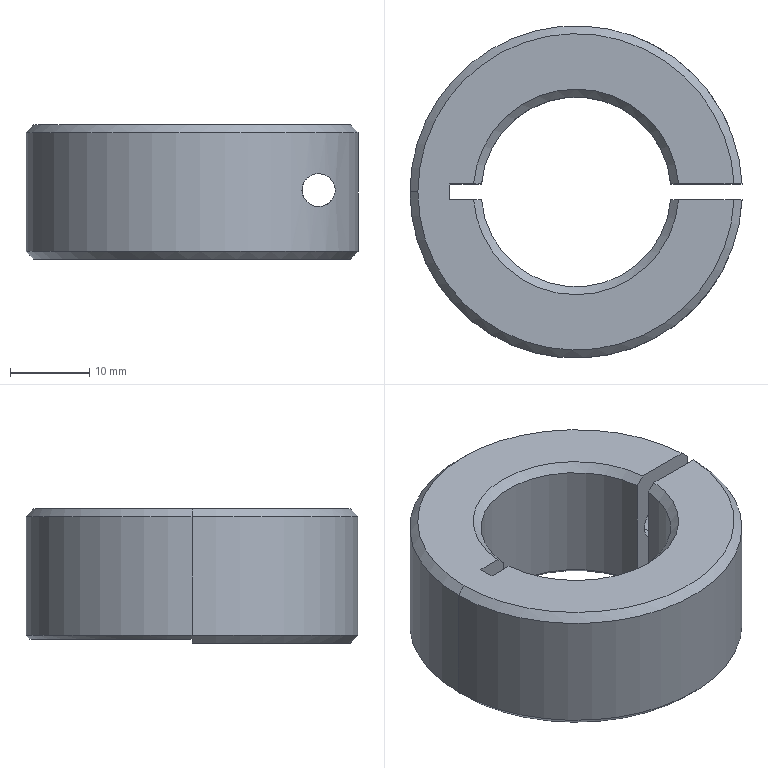Part | SolidWorks | features ICE 7, Chamfer 2, HoleWzd 2 | 1 solid | 44 faces | box 41.976 x 42 x 17 mm | volume 13853 mm3 | cylinder 18 | cone 13 | plane 13 | commonest cylinder face diameters 3.3 x6 14 x3 4.2 x2 5.5 x2 24 x2 42 x2
STEP:
#1=CARTESIAN_POINT('',(15.988,13.615,1.75));
#2=VERTEX_POINT('',#1);
#3=CARTESIAN_POINT('',(15.988,13.615,15.75));
#4=VERTEX_POINT('',#3);
#5=CARTESIAN_POINT('',(15.988,13.615,1.75));
#6=CARTESIAN_POINT('',(15.646,14.017,1.75));
#7=CARTESIAN_POINT('',(15.292,14.403,1.775));
#8=CARTESIAN_POINT('',(14.558,15.144,1.888));
#9=CARTESIAN_POINT('',(14.178,15.5,1.976));
#10=CARTESIAN_POINT('',(13.402,16.176,2.232));
#11=CARTESIAN_POINT('',(13.014,16.489,2.398));
#12=CARTESIAN_POINT('',(12.437,16.923,2.714));
#13=CARTESIAN_POINT('',(12.245,17.062,2.83));
#14=CARTESIAN_POINT('',(11.866,17.328,3.088));
#15=CARTESIAN_POINT('',(11.678,17.455,3.229));
#16=CARTESIAN_POINT('',(11.137,17.809,3.681));
#17=CARTESIAN_POINT('',(10.8,18.013,4.024));
#18=CARTESIAN_POINT('',(10.34,18.279,4.608));
#19=CARTESIAN_POINT('',(10.193,18.361,4.815));
#20=CARTESIAN_POINT('',(9.922,18.509,5.247));
#21=CARTESIAN_POINT('',(9.799,18.574,5.47));
#22=CARTESIAN_POINT('',(9.576,18.69,5.931));
#23=CARTESIAN_POINT('',(9.476,18.74,6.168));
#24=CARTESIAN_POINT('',(9.303,18.827,6.658));
#25=CARTESIAN_POINT('',(9.229,18.864,6.912));
#26=CARTESIAN_POINT('',(9.05,18.95,7.683));
#27=CARTESIAN_POINT('',(8.989,18.979,8.204));
#28=CARTESIAN_POINT('',(8.987,18.98,8.998));
#29=CARTESIAN_POINT('',(9.002,18.973,9.266));
#30=CARTESIAN_POINT('',(9.061,18.945,9.791));
#31=CARTESIAN_POINT('',(9.105,18.924,10.049));
#32=CARTESIAN_POINT('',(9.221,18.867,10.559));
#33=CARTESIAN_POINT('',(9.293,18.832,10.811));
#34=CARTESIAN_POINT('',(9.466,18.746,11.306));
#35=CARTESIAN_POINT('',(9.566,18.695,11.548));
#36=CARTESIAN_POINT('',(9.9,18.521,12.243));
#37=CARTESIAN_POINT('',(10.17,18.376,12.675));
#38=CARTESIAN_POINT('',(10.789,18.02,13.464));
#39=CARTESIAN_POINT('',(11.129,17.814,13.811));
#40=CARTESIAN_POINT('',(11.672,17.459,14.266));
#41=CARTESIAN_POINT('',(11.86,17.332,14.408));
#42=CARTESIAN_POINT('',(12.239,17.066,14.666));
#43=CARTESIAN_POINT('',(12.43,16.928,14.783));
#44=CARTESIAN_POINT('',(12.816,16.637,14.994));
#45=CARTESIAN_POINT('',(13.01,16.486,15.089));
#46=CARTESIAN_POINT('',(13.4,16.171,15.257));
#47=CARTESIAN_POINT('',(13.596,16.006,15.332));
#48=CARTESIAN_POINT('',(14.565,15.163,15.652));
#49=CARTESIAN_POINT('',(15.301,14.422,15.75));
#50=CARTESIAN_POINT('',(15.988,13.615,15.75));
#51=B_SPLINE_CURVE_WITH_KNOTS('',3,(#5,#6,#7,#8,#9,#10,#11,#12,#13,#14,#15,#16,#17,#18,#19,#20,#21,#22,#23,#24,#25,#26,#27,#28,#29,#30,#31,#32,#33,#34,#35,#36,#37,#38,#39,#40,#41,#42,#43,#44,#45,#46,#47,#48,#49,#50),.UNSPECIFIED.,.F.,.F.,(4,2,2,2,2,2,2,2,2,2,2,2,2,2,2,2,2,2,2,2,2,2,4),(0.0005356,0.002108,0.00368,0.005253,0.006039,0.006825,0.008398,0.009184,0.00997,0.01076,0.01154,0.01311,0.0139,0.01469,0.01547,0.01626,0.01783,0.0194,0.02019,0.02098,0.02176,0.02255,0.02569),.UNSPECIFIED.);
#52=EDGE_CURVE('',#2,#4,#51,.T.);
#53=ORIENTED_EDGE('',*,*,#52,.T.);
#54=CARTESIAN_POINT('',(15.988,13.2,15.75));
#55=VERTEX_POINT('',#54);
#56=CARTESIAN_POINT('',(15.988,30.2,15.75));
#57=DIRECTION('',(0.,-1.,0.));
#58=VECTOR('',#57,1000.);
#59=LINE('',#56,#58);
#60=EDGE_CURVE('',#4,#55,#59,.T.);
#61=ORIENTED_EDGE('',*,*,#60,.T.);
#62=CARTESIAN_POINT('',(15.988,13.2,1.75));
#63=VERTEX_POINT('',#62);
#64=CARTESIAN_POINT('',(15.988,13.2,8.75));
#65=DIRECTION('',(0.,1.,0.));
#66=DIRECTION('',(0.,0.,1.));
#67=AXIS2_PLACEMENT_3D('',#64,#65,#66);
#68=CIRCLE('',#67,7.);
#69=EDGE_CURVE('',#63,#55,#68,.T.);
#70=ORIENTED_EDGE('',*,*,#69,.F.);
#71=CARTESIAN_POINT('',(15.988,30.2,1.75));
#72=DIRECTION('',(0.,-1.,0.));
#73=VECTOR('',#72,1000.);
#74=LINE('',#71,#73);
#75=EDGE_CURVE('',#2,#63,#74,.T.);
#76=ORIENTED_EDGE('',*,*,#75,.F.);
#77=EDGE_LOOP('',(#53,#61,#70,#76));
#78=FACE_OUTER_BOUND('',#77,.T.);
#79=CARTESIAN_POINT('',(15.988,30.2,8.75));
#80=DIRECTION('',(0.,-1.,0.));
#81=DIRECTION('',(0.,0.,-1.));
#82=AXIS2_PLACEMENT_3D('',#79,#80,#81);
#83=CYLINDRICAL_SURFACE('',#82,7.);
#84=ADVANCED_FACE('',(#78),#83,.F.);
#85=CARTESIAN_POINT('',(16.333,13.2,1.758));
#86=VERTEX_POINT('',#85);
#87=CARTESIAN_POINT('',(16.333,13.2,1.758));
#88=CARTESIAN_POINT('',(16.219,13.34,1.753));
#89=CARTESIAN_POINT('',(16.104,13.479,1.75));
#90=CARTESIAN_POINT('',(15.988,13.615,1.75));
#91=B_SPLINE_CURVE_WITH_KNOTS('',3,(#87,#88,#89,#90),.UNSPECIFIED.,.F.,.F.,(4,4),(0.,0.0005356),.UNSPECIFIED.);
#92=EDGE_CURVE('',#86,#2,#91,.T.);
#93=ORIENTED_EDGE('',*,*,#92,.T.);
#94=ORIENTED_EDGE('',*,*,#75,.T.);
#95=CARTESIAN_POINT('',(15.988,13.2,8.75));
#96=DIRECTION('',(0.,1.,0.));
#97=DIRECTION('',(0.,0.,1.));
#98=AXIS2_PLACEMENT_3D('',#95,#96,#97);
#99=CIRCLE('',#98,7.);
#100=EDGE_CURVE('',#86,#63,#99,.T.);
#101=ORIENTED_EDGE('',*,*,#100,.F.);
#102=EDGE_LOOP('',(#93,#94,#101));
#103=FACE_OUTER_BOUND('',#102,.T.);
#104=CARTESIAN_POINT('',(15.988,30.2,8.75));
#105=DIRECTION('',(0.,-1.,0.));
#106=DIRECTION('',(0.,0.,-1.));
#107=AXIS2_PLACEMENT_3D('',#104,#105,#106);
#108=CYLINDRICAL_SURFACE('',#107,7.);
#109=ADVANCED_FACE('',(#103),#108,.F.);
#110=CARTESIAN_POINT('',(-14.795,-5.985,10.1));
#111=VERTEX_POINT('',#110);
#112=CARTESIAN_POINT('',(-18.095,-5.985,10.1));
#113=VERTEX_POINT('',#112);
#114=CARTESIAN_POINT('',(-16.445,-5.985,10.1));
#115=DIRECTION('',(0.,0.,-1.));
#116=DIRECTION('',(-1.,0.,0.));
#117=AXIS2_PLACEMENT_3D('',#114,#115,#116);
#118=CIRCLE('',#117,1.65);
#119=EDGE_CURVE('',#111,#113,#118,.T.);
#120=ORIENTED_EDGE('',*,*,#119,.F.);
#121=CARTESIAN_POINT('',(-14.795,-5.985,0.));
#122=VERTEX_POINT('',#121);
#123=CARTESIAN_POINT('',(-14.795,-5.985,0.));
#124=DIRECTION('',(0.,0.,-1.));
#125=VECTOR('',#124,1000.);
#126=LINE('',#123,#125);
#127=EDGE_CURVE('',#111,#122,#126,.T.);
#128=ORIENTED_EDGE('',*,*,#127,.T.);
#129=CARTESIAN_POINT('',(-18.095,-5.985,0.));
#130=VERTEX_POINT('',#129);
#131=CARTESIAN_POINT('',(-16.445,-5.985,0.));
#132=DIRECTION('',(0.,0.,-1.));
#133=DIRECTION('',(-1.,0.,0.));
#134=AXIS2_PLACEMENT_3D('',#131,#132,#133);
#135=CIRCLE('',#134,1.65);
#136=EDGE_CURVE('',#122,#130,#135,.T.);
#137=ORIENTED_EDGE('',*,*,#136,.T.);
#138=CARTESIAN_POINT('',(-18.095,-5.985,0.));
#139=DIRECTION('',(0.,0.,-1.));
#140=VECTOR('',#139,1000.);
#141=LINE('',#138,#140);
#142=EDGE_CURVE('',#113,#130,#141,.T.);
#143=ORIENTED_EDGE('',*,*,#142,.F.);
#144=EDGE_LOOP('',(#120,#128,#137,#143));
#145=FACE_OUTER_BOUND('',#144,.T.);
#146=CARTESIAN_POINT('',(-16.445,-5.985,0.));
#147=DIRECTION('',(0.,0.,-1.));
#148=DIRECTION('',(-1.,0.,0.));
#149=AXIS2_PLACEMENT_3D('',#146,#147,#148);
#150=CYLINDRICAL_SURFACE('',#149,1.65);
#151=ADVANCED_FACE('',(#145),#150,.F.);
#152=CARTESIAN_POINT('',(-16.445,-5.985,11.091));
#153=VERTEX_POINT('',#152);
#154=CARTESIAN_POINT('',(-18.095,-5.985,10.1));
#155=DIRECTION('',(-0.8572,0.,-0.515));
#156=VECTOR('',#155,1000.);
#157=LINE('',#154,#156);
#158=EDGE_CURVE('',#153,#113,#157,.T.);
#159=ORIENTED_EDGE('',*,*,#158,.F.);
#160=CARTESIAN_POINT('',(-14.795,-5.985,10.1));
#161=DIRECTION('',(0.8572,0.,-0.515));
#162=VECTOR('',#161,1000.);
#163=LINE('',#160,#162);
#164=EDGE_CURVE('',#153,#111,#163,.T.);
#165=ORIENTED_EDGE('',*,*,#164,.T.);
#166=ORIENTED_EDGE('',*,*,#119,.T.);
#167=EDGE_LOOP('',(#159,#165,#166));
#168=FACE_OUTER_BOUND('',#167,.T.);
#169=CARTESIAN_POINT('',(-16.445,-5.985,10.1));
#170=DIRECTION('',(0.,0.,-1.));
#171=DIRECTION('',(-1.,0.,0.));
#172=AXIS2_PLACEMENT_3D('',#169,#170,#171);
#173=CONICAL_SURFACE('',#172,1.65,1.03);
#174=ADVANCED_FACE('',(#168),#173,.F.);
#175=CARTESIAN_POINT('',(10.4,-15.155,10.1));
#176=VERTEX_POINT('',#175);
#177=CARTESIAN_POINT('',(7.1,-15.155,10.1));
#178=VERTEX_POINT('',#177);
#179=CARTESIAN_POINT('',(8.75,-15.155,10.1));
#180=DIRECTION('',(0.,0.,-1.));
#181=DIRECTION('',(-1.,0.,0.));
#182=AXIS2_PLACEMENT_3D('',#179,#180,#181);
#183=CIRCLE('',#182,1.65);
#184=EDGE_CURVE('',#176,#178,#183,.T.);
#185=ORIENTED_EDGE('',*,*,#184,.F.);
#186=CARTESIAN_POINT('',(10.4,-15.155,0.));
#187=VERTEX_POINT('',#186);
#188=CARTESIAN_POINT('',(10.4,-15.155,0.));
#189=DIRECTION('',(0.,0.,-1.));
#190=VECTOR('',#189,1000.);
#191=LINE('',#188,#190);
#192=EDGE_CURVE('',#176,#187,#191,.T.);
#193=ORIENTED_EDGE('',*,*,#192,.T.);
#194=CARTESIAN_POINT('',(7.1,-15.155,0.));
#195=VERTEX_POINT('',#194);
#196=CARTESIAN_POINT('',(8.75,-15.155,0.));
#197=DIRECTION('',(0.,0.,-1.));
#198=DIRECTION('',(-1.,0.,0.));
#199=AXIS2_PLACEMENT_3D('',#196,#197,#198);
#200=CIRCLE('',#199,1.65);
#201=EDGE_CURVE('',#187,#195,#200,.T.);
#202=ORIENTED_EDGE('',*,*,#201,.T.);
#203=CARTESIAN_POINT('',(7.1,-15.155,0.));
#204=DIRECTION('',(0.,0.,-1.));
#205=VECTOR('',#204,1000.);
#206=LINE('',#203,#205);
#207=EDGE_CURVE('',#178,#195,#206,.T.);
#208=ORIENTED_EDGE('',*,*,#207,.F.);
#209=EDGE_LOOP('',(#185,#193,#202,#208));
#210=FACE_OUTER_BOUND('',#209,.T.);
#211=CARTESIAN_POINT('',(8.75,-15.155,0.));
#212=DIRECTION('',(0.,0.,-1.));
#213=DIRECTION('',(-1.,0.,0.));
#214=AXIS2_PLACEMENT_3D('',#211,#212,#213);
#215=CYLINDRICAL_SURFACE('',#214,1.65);
#216=ADVANCED_FACE('',(#210),#215,.F.);
#217=CARTESIAN_POINT('',(8.75,-15.155,11.091));
#218=VERTEX_POINT('',#217);
#219=CARTESIAN_POINT('',(7.1,-15.155,10.1));
#220=DIRECTION('',(-0.8572,0.,-0.515));
#221=VECTOR('',#220,1000.);
#222=LINE('',#219,#221);
#223=EDGE_CURVE('',#218,#178,#222,.T.);
#224=ORIENTED_EDGE('',*,*,#223,.F.);
#225=CARTESIAN_POINT('',(10.4,-15.155,10.1));
#226=DIRECTION('',(0.8572,0.,-0.515));
#227=VECTOR('',#226,1000.);
#228=LINE('',#225,#227);
#229=EDGE_CURVE('',#218,#176,#228,.T.);
#230=ORIENTED_EDGE('',*,*,#229,.T.);
#231=ORIENTED_EDGE('',*,*,#184,.T.);
#232=EDGE_LOOP('',(#224,#230,#231));
#233=FACE_OUTER_BOUND('',#232,.T.);
#234=CARTESIAN_POINT('',(8.75,-15.155,10.1));
#235=DIRECTION('',(0.,0.,-1.));
#236=DIRECTION('',(-1.,0.,0.));
#237=AXIS2_PLACEMENT_3D('',#234,#235,#236);
#238=CONICAL_SURFACE('',#237,1.65,1.03);
#239=ADVANCED_FACE('',(#233),#238,.F.);
#240=CARTESIAN_POINT('',(-4.335,-16.445,10.1));
#241=VERTEX_POINT('',#240);
#242=CARTESIAN_POINT('',(-7.635,-16.445,10.1));
#243=VERTEX_POINT('',#242);
#244=CARTESIAN_POINT('',(-5.985,-16.445,10.1));
#245=DIRECTION('',(0.,0.,-1.));
#246=DIRECTION('',(-1.,0.,0.));
#247=AXIS2_PLACEMENT_3D('',#244,#245,#246);
#248=CIRCLE('',#247,1.65);
#249=EDGE_CURVE('',#241,#243,#248,.T.);
#250=ORIENTED_EDGE('',*,*,#249,.F.);
#251=CARTESIAN_POINT('',(-4.335,-16.445,0.));
#252=VERTEX_POINT('',#251);
#253=CARTESIAN_POINT('',(-4.335,-16.445,0.));
#254=DIRECTION('',(0.,0.,-1.));
#255=VECTOR('',#254,1000.);
#256=LINE('',#253,#255);
#257=EDGE_CURVE('',#241,#252,#256,.T.);
#258=ORIENTED_EDGE('',*,*,#257,.T.);
#259=CARTESIAN_POINT('',(-7.635,-16.445,0.));
#260=VERTEX_POINT('',#259);
#261=CARTESIAN_POINT('',(-5.985,-16.445,0.));
#262=DIRECTION('',(0.,0.,-1.));
#263=DIRECTION('',(-1.,0.,0.));
#264=AXIS2_PLACEMENT_3D('',#261,#262,#263);
#265=CIRCLE('',#264,1.65);
#266=EDGE_CURVE('',#252,#260,#265,.T.);
#267=ORIENTED_EDGE('',*,*,#266,.T.);
#268=CARTESIAN_POINT('',(-7.635,-16.445,0.));
#269=DIRECTION('',(0.,0.,-1.));
#270=VECTOR('',#269,1000.);
#271=LINE('',#268,#270);
#272=EDGE_CURVE('',#243,#260,#271,.T.);
#273=ORIENTED_EDGE('',*,*,#272,.F.);
#274=EDGE_LOOP('',(#250,#258,#267,#273));
#275=FACE_OUTER_BOUND('',#274,.T.);
#276=CARTESIAN_POINT('',(-5.985,-16.445,0.));
#277=DIRECTION('',(0.,0.,-1.));
#278=DIRECTION('',(-1.,0.,0.));
#279=AXIS2_PLACEMENT_3D('',#276,#277,#278);
#280=CYLINDRICAL_SURFACE('',#279,1.65);
#281=ADVANCED_FACE('',(#275),#280,.F.);
#282=CARTESIAN_POINT('',(-5.985,-16.445,11.091));
#283=VERTEX_POINT('',#282);
#284=CARTESIAN_POINT('',(-7.635,-16.445,10.1));
#285=DIRECTION('',(-0.8572,0.,-0.515));
#286=VECTOR('',#285,1000.);
#287=LINE('',#284,#286);
#288=EDGE_CURVE('',#283,#243,#287,.T.);
#289=ORIENTED_EDGE('',*,*,#288,.F.);
#290=CARTESIAN_POINT('',(-4.335,-16.445,10.1));
#291=DIRECTION('',(0.8572,0.,-0.515));
#292=VECTOR('',#291,1000.);
#293=LINE('',#290,#292);
#294=EDGE_CURVE('',#283,#241,#293,.T.);
#295=ORIENTED_EDGE('',*,*,#294,.T.);
#296=ORIENTED_EDGE('',*,*,#249,.T.);
#297=EDGE_LOOP('',(#289,#295,#296));
#298=FACE_OUTER_BOUND('',#297,.T.);
#299=CARTESIAN_POINT('',(-5.985,-16.445,10.1));
#300=DIRECTION('',(0.,0.,-1.));
#301=DIRECTION('',(-1.,0.,0.));
#302=AXIS2_PLACEMENT_3D('',#299,#300,#301);
#303=CONICAL_SURFACE('',#302,1.65,1.03);
#304=ADVANCED_FACE('',(#298),#303,.F.);
#305=CARTESIAN_POINT('',(15.988,-13.615,6.65));
#306=VERTEX_POINT('',#305);
#307=CARTESIAN_POINT('',(15.988,-13.615,10.85));
#308=VERTEX_POINT('',#307);
#309=CARTESIAN_POINT('',(15.988,-13.615,6.65));
#310=CARTESIAN_POINT('',(15.769,-13.873,6.65));
#311=CARTESIAN_POINT('',(15.546,-14.122,6.683));
#312=CARTESIAN_POINT('',(15.21,-14.481,6.796));
#313=CARTESIAN_POINT('',(15.096,-14.599,6.845));
#314=CARTESIAN_POINT('',(14.875,-14.824,6.965));
#315=CARTESIAN_POINT('',(14.767,-14.931,7.036));
#316=CARTESIAN_POINT('',(14.454,-15.237,7.291));
#317=CARTESIAN_POINT('',(14.26,-15.417,7.516));
#318=CARTESIAN_POINT('',(14.046,-15.611,7.935));
#319=CARTESIAN_POINT('',(13.989,-15.662,8.085));
#320=CARTESIAN_POINT('',(13.909,-15.733,8.41));
#321=CARTESIAN_POINT('',(13.888,-15.752,8.576));
#322=CARTESIAN_POINT('',(13.888,-15.752,8.915));
#323=CARTESIAN_POINT('',(13.908,-15.734,9.085));
#324=CARTESIAN_POINT('',(13.987,-15.664,9.407));
#325=CARTESIAN_POINT('',(14.045,-15.613,9.561));
#326=CARTESIAN_POINT('',(14.187,-15.484,9.84));
#327=CARTESIAN_POINT('',(14.271,-15.406,9.968));
#328=CARTESIAN_POINT('',(14.455,-15.234,10.192));
#329=CARTESIAN_POINT('',(14.555,-15.138,10.291));
#330=CARTESIAN_POINT('',(14.87,-14.832,10.548));
#331=CARTESIAN_POINT('',(15.092,-14.606,10.664));
#332=CARTESIAN_POINT('',(15.544,-14.124,10.816));
#333=CARTESIAN_POINT('',(15.768,-13.874,10.85));
#334=CARTESIAN_POINT('',(15.988,-13.615,10.85));
#335=B_SPLINE_CURVE_WITH_KNOTS('',3,(#309,#310,#311,#312,#313,#314,#315,#316,#317,#318,#319,#320,#321,#322,#323,#324,#325,#326,#327,#328,#329,#330,#331,#332,#333,#334),.UNSPECIFIED.,.F.,.F.,(4,2,2,2,2,2,2,2,2,2,2,2,4),(0.009008,0.01001,0.01052,0.01102,0.01202,0.01253,0.01303,0.01353,0.01403,0.01453,0.01504,0.01604,0.01705),.UNSPECIFIED.);
#336=EDGE_CURVE('',#306,#308,#335,.T.);
#337=ORIENTED_EDGE('',*,*,#336,.F.);
#338=CARTESIAN_POINT('',(15.988,-1.,6.65));
#339=VERTEX_POINT('',#338);
#340=CARTESIAN_POINT('',(15.988,-1.,6.65));
#341=DIRECTION('',(0.,1.,0.));
#342=VECTOR('',#341,1000.);
#343=LINE('',#340,#342);
#344=EDGE_CURVE('',#306,#339,#343,.T.);
#345=ORIENTED_EDGE('',*,*,#344,.T.);
#346=CARTESIAN_POINT('',(15.988,-1.,10.85));
#347=VERTEX_POINT('',#346);
#348=CARTESIAN_POINT('',(15.988,-1.,8.75));
#349=DIRECTION('',(0.,1.,0.));
#350=DIRECTION('',(0.,0.,1.));
#351=AXIS2_PLACEMENT_3D('',#348,#349,#350);
#352=CIRCLE('',#351,2.1);
#353=EDGE_CURVE('',#339,#347,#352,.T.);
#354=ORIENTED_EDGE('',*,*,#353,.T.);
#355=CARTESIAN_POINT('',(15.988,-1.,10.85));
#356=DIRECTION('',(0.,1.,0.));
#357=VECTOR('',#356,1000.);
#358=LINE('',#355,#357);
#359=EDGE_CURVE('',#308,#347,#358,.T.);
#360=ORIENTED_EDGE('',*,*,#359,.F.);
#361=EDGE_LOOP('',(#337,#345,#354,#360));
#362=FACE_OUTER_BOUND('',#361,.T.);
#363=CARTESIAN_POINT('',(15.988,-1.,8.75));
#364=DIRECTION('',(0.,1.,0.));
#365=DIRECTION('',(0.,0.,1.));
#366=AXIS2_PLACEMENT_3D('',#363,#364,#365);
#367=CYLINDRICAL_SURFACE('',#366,2.1);
#368=ADVANCED_FACE('',(#362),#367,.F.);
#369=CARTESIAN_POINT('',(15.988,9.,6.));
#370=VERTEX_POINT('',#369);
#371=CARTESIAN_POINT('',(15.988,9.,11.5));
#372=VERTEX_POINT('',#371);
#373=CARTESIAN_POINT('',(15.988,9.,8.75));
#374=DIRECTION('',(0.,1.,0.));
#375=DIRECTION('',(0.,0.,-1.));
#376=AXIS2_PLACEMENT_3D('',#373,#374,#375);
#377=CIRCLE('',#376,2.75);
#378=EDGE_CURVE('',#370,#372,#377,.T.);
#379=ORIENTED_EDGE('',*,*,#378,.T.);
#380=CARTESIAN_POINT('',(15.988,1.,11.5));
#381=VERTEX_POINT('',#380);
#382=CARTESIAN_POINT('',(15.988,31.,11.5));
#383=DIRECTION('',(0.,-1.,0.));
#384=VECTOR('',#383,1000.);
#385=LINE('',#382,#384);
#386=EDGE_CURVE('',#372,#381,#385,.T.);
#387=ORIENTED_EDGE('',*,*,#386,.T.);
#388=CARTESIAN_POINT('',(15.988,1.,6.));
#389=VERTEX_POINT('',#388);
#390=CARTESIAN_POINT('',(15.988,1.,8.75));
#391=DIRECTION('',(0.,-1.,0.));
#392=DIRECTION('',(0.,0.,-1.));
#393=AXIS2_PLACEMENT_3D('',#390,#391,#392);
#394=CIRCLE('',#393,2.75);
#395=EDGE_CURVE('',#381,#389,#394,.T.);
#396=ORIENTED_EDGE('',*,*,#395,.T.);
#397=CARTESIAN_POINT('',(15.988,31.,6.));
#398=DIRECTION('',(0.,-1.,0.));
#399=VECTOR('',#398,1000.);
#400=LINE('',#397,#399);
#401=EDGE_CURVE('',#370,#389,#400,.T.);
#402=ORIENTED_EDGE('',*,*,#401,.F.);
#403=EDGE_LOOP('',(#379,#387,#396,#402));
#404=FACE_OUTER_BOUND('',#403,.T.);
#405=CARTESIAN_POINT('',(15.988,31.,8.75));
#406=DIRECTION('',(0.,-1.,0.));
#407=DIRECTION('',(0.,0.,-1.));
#408=AXIS2_PLACEMENT_3D('',#405,#406,#407);
#409=CYLINDRICAL_SURFACE('',#408,2.75);
#410=ADVANCED_FACE('',(#404),#409,.F.);
#411=CARTESIAN_POINT('',(-20.,0.,17.));
#412=VERTEX_POINT('',#411);
#413=CARTESIAN_POINT('',(19.975,-1.,17.));
#414=VERTEX_POINT('',#413);
#415=CARTESIAN_POINT('',(0.,0.,17.));
#416=DIRECTION('',(0.,0.,1.));
#417=DIRECTION('',(1.,0.,0.));
#418=AXIS2_PLACEMENT_3D('',#415,#416,#417);
#419=CIRCLE('',#418,20.);
#420=EDGE_CURVE('',#412,#414,#419,.T.);
#421=ORIENTED_EDGE('',*,*,#420,.F.);
#422=CARTESIAN_POINT('',(-21.,0.,16.));
#423=VERTEX_POINT('',#422);
#424=CARTESIAN_POINT('',(-20.,0.,17.));
#425=DIRECTION('',(-0.7071,0.,-0.7071));
#426=VECTOR('',#425,1000.);
#427=LINE('',#424,#426);
#428=EDGE_CURVE('',#412,#423,#427,.T.);
#429=ORIENTED_EDGE('',*,*,#428,.T.);
#430=CARTESIAN_POINT('',(20.976,-1.,16.));
#431=VERTEX_POINT('',#430);
#432=CARTESIAN_POINT('',(0.,0.,16.));
#433=DIRECTION('',(0.,0.,-1.));
#434=DIRECTION('',(1.,0.,0.));
#435=AXIS2_PLACEMENT_3D('',#432,#433,#434);
#436=CIRCLE('',#435,21.);
#437=EDGE_CURVE('',#431,#423,#436,.T.);
#438=ORIENTED_EDGE('',*,*,#437,.F.);
#439=CARTESIAN_POINT('',(19.975,-1.,17.));
#440=CARTESIAN_POINT('',(20.309,-1.,16.667));
#441=CARTESIAN_POINT('',(20.642,-1.,16.333));
#442=CARTESIAN_POINT('',(20.976,-1.,16.));
#443=B_SPLINE_CURVE_WITH_KNOTS('',3,(#439,#440,#441,#442),.UNSPECIFIED.,.F.,.F.,(4,4),(0.08115,0.08257),.UNSPECIFIED.);
#444=EDGE_CURVE('',#414,#431,#443,.T.);
#445=ORIENTED_EDGE('',*,*,#444,.F.);
#446=EDGE_LOOP('',(#421,#429,#438,#445));
#447=FACE_OUTER_BOUND('',#446,.T.);
#448=CARTESIAN_POINT('',(0.,0.,17.));
#449=DIRECTION('',(0.,0.,-1.));
#450=DIRECTION('',(-1.,0.,0.));
#451=AXIS2_PLACEMENT_3D('',#448,#449,#450);
#452=CONICAL_SURFACE('',#451,20.,0.7854);
#453=ADVANCED_FACE('',(#447),#452,.T.);
#454=CARTESIAN_POINT('',(15.988,-13.615,10.85));
#455=CARTESIAN_POINT('',(16.235,-13.326,10.85));
#456=CARTESIAN_POINT('',(16.469,-13.035,10.808));
#457=CARTESIAN_POINT('',(16.915,-12.451,10.649));
#458=CARTESIAN_POINT('',(17.129,-12.154,10.531));
#459=CARTESIAN_POINT('',(17.419,-11.731,10.292));
#460=CARTESIAN_POINT('',(17.511,-11.593,10.202));
#461=CARTESIAN_POINT('',(17.685,-11.326,9.995));
#462=CARTESIAN_POINT('',(17.766,-11.198,9.878));
#463=CARTESIAN_POINT('',(17.909,-10.968,9.612));
#464=CARTESIAN_POINT('',(17.971,-10.865,9.462));
#465=CARTESIAN_POINT('',(18.062,-10.714,9.125));
#466=CARTESIAN_POINT('',(18.089,-10.668,8.935));
#467=CARTESIAN_POINT('',(18.088,-10.67,8.554));
#468=CARTESIAN_POINT('',(18.06,-10.717,8.366));
#469=CARTESIAN_POINT('',(17.969,-10.869,8.031));
#470=CARTESIAN_POINT('',(17.906,-10.973,7.881));
#471=CARTESIAN_POINT('',(17.763,-11.203,7.617));
#472=CARTESIAN_POINT('',(17.681,-11.332,7.5));
#473=CARTESIAN_POINT('',(17.508,-11.597,7.295));
#474=CARTESIAN_POINT('',(17.416,-11.735,7.205));
#475=CARTESIAN_POINT('',(17.223,-12.016,7.047));
#476=CARTESIAN_POINT('',(17.121,-12.161,6.978));
#477=CARTESIAN_POINT('',(16.91,-12.453,6.86));
#478=CARTESIAN_POINT('',(16.802,-12.598,6.811));
#479=CARTESIAN_POINT('',(16.469,-13.035,6.692));
#480=CARTESIAN_POINT('',(16.234,-13.327,6.65));
#481=CARTESIAN_POINT('',(15.988,-13.615,6.65));
#482=B_SPLINE_CURVE_WITH_KNOTS('',3,(#454,#455,#456,#457,#458,#459,#460,#461,#462,#463,#464,#465,#466,#467,#468,#469,#470,#471,#472,#473,#474,#475,#476,#477,#478,#479,#480,#481),.UNSPECIFIED.,.F.,.F.,(4,2,2,2,2,2,2,2,2,2,2,2,2,4),(0.,0.001126,0.002252,0.002815,0.003378,0.003941,0.004504,0.005067,0.00563,0.006193,0.006756,0.007319,0.007882,0.009008),.UNSPECIFIED.);
#483=EDGE_CURVE('',#308,#306,#482,.T.);
#484=ORIENTED_EDGE('',*,*,#483,.T.);
#485=ORIENTED_EDGE('',*,*,#336,.T.);
#486=EDGE_LOOP('',(#484,#485));
#487=FACE_BOUND('',#486,.T.);
#488=ORIENTED_EDGE('',*,*,#437,.T.);
#489=CARTESIAN_POINT('',(-21.,0.,1.));
#490=VERTEX_POINT('',#489);
#491=CARTESIAN_POINT('',(-21.,0.,17.));
#492=DIRECTION('',(0.,0.,-1.));
#493=VECTOR('',#492,1000.);
#494=LINE('',#491,#493);
#495=EDGE_CURVE('',#423,#490,#494,.T.);
#496=ORIENTED_EDGE('',*,*,#495,.T.);
#497=CARTESIAN_POINT('',(20.976,-1.,1.));
#498=VERTEX_POINT('',#497);
#499=CARTESIAN_POINT('',(0.,0.,1.));
#500=DIRECTION('',(0.,0.,1.));
#501=DIRECTION('',(1.,0.,0.));
#502=AXIS2_PLACEMENT_3D('',#499,#500,#501);
#503=CIRCLE('',#502,21.);
#504=EDGE_CURVE('',#490,#498,#503,.T.);
#505=ORIENTED_EDGE('',*,*,#504,.T.);
#506=CARTESIAN_POINT('',(20.976,-1.,17.));
#507=DIRECTION('',(0.,0.,1.));
#508=VECTOR('',#507,1000.);
#509=LINE('',#506,#508);
#510=EDGE_CURVE('',#498,#431,#509,.T.);
#511=ORIENTED_EDGE('',*,*,#510,.T.);
#512=EDGE_LOOP('',(#488,#496,#505,#511));
#513=FACE_OUTER_BOUND('',#512,.T.);
#514=CARTESIAN_POINT('',(0.,0.,17.));
#515=DIRECTION('',(0.,0.,-1.));
#516=DIRECTION('',(-1.,0.,0.));
#517=AXIS2_PLACEMENT_3D('',#514,#515,#516);
#518=CYLINDRICAL_SURFACE('',#517,21.);
#519=ADVANCED_FACE('',(#487,#513),#518,.T.);
#520=ORIENTED_EDGE('',*,*,#495,.F.);
#521=CARTESIAN_POINT('',(20.976,1.,16.));
#522=VERTEX_POINT('',#521);
#523=CARTESIAN_POINT('',(0.,0.,16.));
#524=DIRECTION('',(0.,0.,-1.));
#525=DIRECTION('',(1.,0.,0.));
#526=AXIS2_PLACEMENT_3D('',#523,#524,#525);
#527=CIRCLE('',#526,21.);
#528=EDGE_CURVE('',#423,#522,#527,.T.);
#529=ORIENTED_EDGE('',*,*,#528,.T.);
#530=CARTESIAN_POINT('',(20.976,1.,1.));
#531=VERTEX_POINT('',#530);
#532=CARTESIAN_POINT('',(20.976,1.,17.));
#533=DIRECTION('',(0.,0.,-1.));
#534=VECTOR('',#533,1000.);
#535=LINE('',#532,#534);
#536=EDGE_CURVE('',#522,#531,#535,.T.);
#537=ORIENTED_EDGE('',*,*,#536,.T.);
#538=CARTESIAN_POINT('',(0.,0.,1.));
#539=DIRECTION('',(0.,0.,1.));
#540=DIRECTION('',(1.,0.,0.));
#541=AXIS2_PLACEMENT_3D('',#538,#539,#540);
#542=CIRCLE('',#541,21.);
#543=EDGE_CURVE('',#531,#490,#542,.T.);
#544=ORIENTED_EDGE('',*,*,#543,.T.);
#545=EDGE_LOOP('',(#520,#529,#537,#544));
#546=FACE_OUTER_BOUND('',#545,.T.);
#547=CARTESIAN_POINT('',(16.333,13.2,15.742));
#548=VERTEX_POINT('',#547);
#549=CARTESIAN_POINT('',(16.333,13.2,14.5));
#550=VERTEX_POINT('',#549);
#551=CARTESIAN_POINT('',(16.333,13.2,17.));
#552=DIRECTION('',(0.,0.,-1.));
#553=VECTOR('',#552,1000.);
#554=LINE('',#551,#553);
#555=EDGE_CURVE('',#548,#550,#554,.T.);
#556=ORIENTED_EDGE('',*,*,#555,.F.);
#557=CARTESIAN_POINT('',(15.988,13.615,15.75));
#558=CARTESIAN_POINT('',(16.105,13.479,15.75));
#559=CARTESIAN_POINT('',(16.22,13.34,15.747));
#560=CARTESIAN_POINT('',(16.333,13.2,15.742));
#561=B_SPLINE_CURVE_WITH_KNOTS('',3,(#557,#558,#559,#560),.UNSPECIFIED.,.F.,.F.,(4,4),(0.02569,0.02623),.UNSPECIFIED.);
#562=EDGE_CURVE('',#4,#548,#561,.T.);
#563=ORIENTED_EDGE('',*,*,#562,.F.);
#564=ORIENTED_EDGE('',*,*,#52,.F.);
#565=ORIENTED_EDGE('',*,*,#92,.F.);
#566=CARTESIAN_POINT('',(16.333,13.2,3.));
#567=VERTEX_POINT('',#566);
#568=CARTESIAN_POINT('',(16.333,13.2,17.));
#569=DIRECTION('',(0.,0.,-1.));
#570=VECTOR('',#569,1000.);
#571=LINE('',#568,#570);
#572=EDGE_CURVE('',#567,#86,#571,.T.);
#573=ORIENTED_EDGE('',*,*,#572,.F.);
#574=CARTESIAN_POINT('',(18.974,9.,3.));
#575=VERTEX_POINT('',#574);
#576=CARTESIAN_POINT('',(0.,0.,3.));
#577=DIRECTION('',(0.,0.,-1.));
#578=DIRECTION('',(-1.,0.,0.));
#579=AXIS2_PLACEMENT_3D('',#576,#577,#578);
#580=CIRCLE('',#579,21.);
#581=EDGE_CURVE('',#567,#575,#580,.T.);
#582=ORIENTED_EDGE('',*,*,#581,.T.);
#583=CARTESIAN_POINT('',(18.974,9.,14.5));
#584=VERTEX_POINT('',#583);
#585=CARTESIAN_POINT('',(18.974,9.,17.));
#586=DIRECTION('',(0.,0.,1.));
#587=VECTOR('',#586,1000.);
#588=LINE('',#585,#587);
#589=EDGE_CURVE('',#575,#584,#588,.T.);
#590=ORIENTED_EDGE('',*,*,#589,.T.);
#591=CARTESIAN_POINT('',(0.,0.,14.5));
#592=DIRECTION('',(0.,0.,1.));
#593=DIRECTION('',(1.,0.,0.));
#594=AXIS2_PLACEMENT_3D('',#591,#592,#593);
#595=CIRCLE('',#594,21.);
#596=EDGE_CURVE('',#584,#550,#595,.T.);
#597=ORIENTED_EDGE('',*,*,#596,.T.);
#598=EDGE_LOOP('',(#556,#563,#564,#565,#573,#582,#590,#597));
#599=FACE_BOUND('',#598,.T.);
#600=CARTESIAN_POINT('',(0.,0.,17.));
#601=DIRECTION('',(0.,0.,-1.));
#602=DIRECTION('',(-1.,0.,0.));
#603=AXIS2_PLACEMENT_3D('',#600,#601,#602);
#604=CYLINDRICAL_SURFACE('',#603,21.);
#605=ADVANCED_FACE('',(#546,#599),#604,.T.);
#606=CARTESIAN_POINT('',(15.988,13.2,3.));
#607=VERTEX_POINT('',#606);
#608=CARTESIAN_POINT('',(20.976,13.2,3.));
#609=DIRECTION('',(1.,0.,0.));
#610=VECTOR('',#609,1000.);
#611=LINE('',#608,#610);
#612=EDGE_CURVE('',#607,#567,#611,.T.);
#613=ORIENTED_EDGE('',*,*,#612,.F.);
#614=CARTESIAN_POINT('',(15.988,9.,3.));
#615=VERTEX_POINT('',#614);
#616=CARTESIAN_POINT('',(15.988,39.,3.));
#617=DIRECTION('',(0.,-1.,0.));
#618=VECTOR('',#617,1000.);
#619=LINE('',#616,#618);
#620=EDGE_CURVE('',#607,#615,#619,.T.);
#621=ORIENTED_EDGE('',*,*,#620,.T.);
#622=CARTESIAN_POINT('',(20.976,9.,3.));
#623=DIRECTION('',(1.,0.,0.));
#624=VECTOR('',#623,1000.);
#625=LINE('',#622,#624);
#626=EDGE_CURVE('',#615,#575,#625,.T.);
#627=ORIENTED_EDGE('',*,*,#626,.T.);
#628=ORIENTED_EDGE('',*,*,#581,.F.);
#629=EDGE_LOOP('',(#613,#621,#627,#628));
#630=FACE_OUTER_BOUND('',#629,.T.);
#631=CARTESIAN_POINT('',(20.976,39.,3.));
#632=DIRECTION('',(0.,0.,-1.));
#633=DIRECTION('',(-1.,0.,0.));
#634=AXIS2_PLACEMENT_3D('',#631,#632,#633);
#635=PLANE('',#634);
#636=ADVANCED_FACE('',(#630),#635,.F.);
#637=CARTESIAN_POINT('',(15.988,13.2,14.5));
#638=VERTEX_POINT('',#637);
#639=CARTESIAN_POINT('',(15.988,13.2,8.75));
#640=DIRECTION('',(0.,-1.,0.));
#641=DIRECTION('',(0.,0.,1.));
#642=AXIS2_PLACEMENT_3D('',#639,#640,#641);
#643=CIRCLE('',#642,5.75);
#644=EDGE_CURVE('',#638,#607,#643,.T.);
#645=ORIENTED_EDGE('',*,*,#644,.F.);
#646=CARTESIAN_POINT('',(15.988,9.,14.5));
#647=VERTEX_POINT('',#646);
#648=CARTESIAN_POINT('',(15.988,39.,14.5));
#649=DIRECTION('',(0.,-1.,0.));
#650=VECTOR('',#649,1000.);
#651=LINE('',#648,#650);
#652=EDGE_CURVE('',#638,#647,#651,.T.);
#653=ORIENTED_EDGE('',*,*,#652,.T.);
#654=CARTESIAN_POINT('',(15.988,9.,8.75));
#655=DIRECTION('',(0.,-1.,0.));
#656=DIRECTION('',(0.,0.,-1.));
#657=AXIS2_PLACEMENT_3D('',#654,#655,#656);
#658=CIRCLE('',#657,5.75);
#659=EDGE_CURVE('',#647,#615,#658,.T.);
#660=ORIENTED_EDGE('',*,*,#659,.T.);
#661=ORIENTED_EDGE('',*,*,#620,.F.);
#662=EDGE_LOOP('',(#645,#653,#660,#661));
#663=FACE_OUTER_BOUND('',#662,.T.);
#664=CARTESIAN_POINT('',(15.988,39.,8.75));
#665=DIRECTION('',(0.,-1.,0.));
#666=DIRECTION('',(0.,0.,-1.));
#667=AXIS2_PLACEMENT_3D('',#664,#665,#666);
#668=CYLINDRICAL_SURFACE('',#667,5.75);
#669=ADVANCED_FACE('',(#663),#668,.F.);
#670=CARTESIAN_POINT('',(15.988,13.2,14.5));
#671=DIRECTION('',(-1.,0.,0.));
#672=VECTOR('',#671,1000.);
#673=LINE('',#670,#672);
#674=EDGE_CURVE('',#550,#638,#673,.T.);
#675=ORIENTED_EDGE('',*,*,#674,.F.);
#676=ORIENTED_EDGE('',*,*,#596,.F.);
#677=CARTESIAN_POINT('',(15.988,9.,14.5));
#678=DIRECTION('',(-1.,0.,0.));
#679=VECTOR('',#678,1000.);
#680=LINE('',#677,#679);
#681=EDGE_CURVE('',#584,#647,#680,.T.);
#682=ORIENTED_EDGE('',*,*,#681,.T.);
#683=ORIENTED_EDGE('',*,*,#652,.F.);
#684=EDGE_LOOP('',(#675,#676,#682,#683));
#685=FACE_OUTER_BOUND('',#684,.T.);
#686=CARTESIAN_POINT('',(15.988,39.,14.5));
#687=DIRECTION('',(0.,0.,1.));
#688=DIRECTION('',(1.,0.,0.));
#689=AXIS2_PLACEMENT_3D('',#686,#687,#688);
#690=PLANE('',#689);
#691=ADVANCED_FACE('',(#685),#690,.F.);
#692=CARTESIAN_POINT('',(11.958,1.,16.));
#693=VERTEX_POINT('',#692);
#694=CARTESIAN_POINT('',(11.958,1.,1.));
#695=VERTEX_POINT('',#694);
#696=CARTESIAN_POINT('',(11.958,1.,17.));
#697=DIRECTION('',(0.,0.,-1.));
#698=VECTOR('',#697,1000.);
#699=LINE('',#696,#698);
#700=EDGE_CURVE('',#693,#695,#699,.T.);
#701=ORIENTED_EDGE('',*,*,#700,.F.);
#702=CARTESIAN_POINT('',(-11.958,1.,16.));
#703=VERTEX_POINT('',#702);
#704=CARTESIAN_POINT('',(0.,0.,16.));
#705=DIRECTION('',(0.,0.,1.));
#706=DIRECTION('',(1.,0.,0.));
#707=AXIS2_PLACEMENT_3D('',#704,#705,#706);
#708=CIRCLE('',#707,12.);
#709=EDGE_CURVE('',#693,#703,#708,.T.);
#710=ORIENTED_EDGE('',*,*,#709,.T.);
#711=CARTESIAN_POINT('',(-11.958,1.,1.));
#712=VERTEX_POINT('',#711);
#713=CARTESIAN_POINT('',(-11.958,1.,17.));
#714=DIRECTION('',(0.,0.,1.));
#715=VECTOR('',#714,1000.);
#716=LINE('',#713,#715);
#717=EDGE_CURVE('',#712,#703,#716,.T.);
#718=ORIENTED_EDGE('',*,*,#717,.F.);
#719=CARTESIAN_POINT('',(0.,0.,1.));
#720=DIRECTION('',(0.,0.,-1.));
#721=DIRECTION('',(1.,0.,0.));
#722=AXIS2_PLACEMENT_3D('',#719,#720,#721);
#723=CIRCLE('',#722,12.);
#724=EDGE_CURVE('',#712,#695,#723,.T.);
#725=ORIENTED_EDGE('',*,*,#724,.T.);
#726=EDGE_LOOP('',(#701,#710,#718,#725));
#727=FACE_OUTER_BOUND('',#726,.T.);
#728=CARTESIAN_POINT('',(0.,0.,17.));
#729=DIRECTION('',(0.,0.,-1.));
#730=DIRECTION('',(-1.,0.,0.));
#731=AXIS2_PLACEMENT_3D('',#728,#729,#730);
#732=CYLINDRICAL_SURFACE('',#731,12.);
#733=ADVANCED_FACE('',(#727),#732,.F.);
#734=CARTESIAN_POINT('',(12.961,1.,17.));
#735=VERTEX_POINT('',#734);
#736=CARTESIAN_POINT('',(12.961,1.,17.));
#737=CARTESIAN_POINT('',(12.627,1.,16.667));
#738=CARTESIAN_POINT('',(12.293,1.,16.333));
#739=CARTESIAN_POINT('',(11.958,1.,16.));
#740=B_SPLINE_CURVE_WITH_KNOTS('',3,(#736,#737,#738,#739),.UNSPECIFIED.,.F.,.F.,(4,4),(0.02209,0.02351),.UNSPECIFIED.);
#741=EDGE_CURVE('',#735,#693,#740,.T.);
#742=ORIENTED_EDGE('',*,*,#741,.F.);
#743=CARTESIAN_POINT('',(-12.961,1.,17.));
#744=VERTEX_POINT('',#743);
#745=CARTESIAN_POINT('',(0.,0.,17.));
#746=DIRECTION('',(0.,0.,-1.));
#747=DIRECTION('',(1.,0.,0.));
#748=AXIS2_PLACEMENT_3D('',#745,#746,#747);
#749=CIRCLE('',#748,13.);
#750=EDGE_CURVE('',#744,#735,#749,.T.);
#751=ORIENTED_EDGE('',*,*,#750,.F.);
#752=CARTESIAN_POINT('',(-11.958,1.,16.));
#753=CARTESIAN_POINT('',(-12.293,1.,16.333));
#754=CARTESIAN_POINT('',(-12.627,1.,16.667));
#755=CARTESIAN_POINT('',(-12.961,1.,17.));
#756=B_SPLINE_CURVE_WITH_KNOTS('',3,(#752,#753,#754,#755),.UNSPECIFIED.,.F.,.F.,(4,4),(0.05622,0.05764),.UNSPECIFIED.);
#757=EDGE_CURVE('',#703,#744,#756,.T.);
#758=ORIENTED_EDGE('',*,*,#757,.F.);
#759=ORIENTED_EDGE('',*,*,#709,.F.);
#760=EDGE_LOOP('',(#742,#751,#758,#759));
#761=FACE_OUTER_BOUND('',#760,.T.);
#762=CARTESIAN_POINT('',(0.,0.,16.));
#763=DIRECTION('',(0.,0.,1.));
#764=DIRECTION('',(1.,0.,0.));
#765=AXIS2_PLACEMENT_3D('',#762,#763,#764);
#766=CONICAL_SURFACE('',#765,12.,0.7854);
#767=ADVANCED_FACE('',(#761),#766,.F.);
#768=CARTESIAN_POINT('',(12.46,1.,0.5));
#769=VERTEX_POINT('',#768);
#770=CARTESIAN_POINT('',(-12.46,1.,0.5));
#771=VERTEX_POINT('',#770);
#772=CARTESIAN_POINT('',(0.,0.,0.5));
#773=DIRECTION('',(0.,0.,1.));
#774=DIRECTION('',(1.,0.,0.));
#775=AXIS2_PLACEMENT_3D('',#772,#773,#774);
#776=CIRCLE('',#775,12.5);
#777=EDGE_CURVE('',#769,#771,#776,.T.);
#778=ORIENTED_EDGE('',*,*,#777,.F.);
#779=CARTESIAN_POINT('',(11.958,1.,1.));
#780=CARTESIAN_POINT('',(12.125,1.,0.8333));
#781=CARTESIAN_POINT('',(12.293,1.,0.6667));
#782=CARTESIAN_POINT('',(12.46,1.,0.5));
#783=B_SPLINE_CURVE_WITH_KNOTS('',3,(#779,#780,#781,#782),.UNSPECIFIED.,.F.,.F.,(4,4),(0.05622,0.05693),.UNSPECIFIED.);
#784=EDGE_CURVE('',#695,#769,#783,.T.);
#785=ORIENTED_EDGE('',*,*,#784,.F.);
#786=ORIENTED_EDGE('',*,*,#724,.F.);
#787=CARTESIAN_POINT('',(-12.46,1.,0.5));
#788=CARTESIAN_POINT('',(-12.293,1.,0.6667));
#789=CARTESIAN_POINT('',(-12.125,1.,0.8333));
#790=CARTESIAN_POINT('',(-11.958,1.,1.));
#791=B_SPLINE_CURVE_WITH_KNOTS('',3,(#787,#788,#789,#790),.UNSPECIFIED.,.F.,.F.,(4,4),(0.0228,0.02351),.UNSPECIFIED.);
#792=EDGE_CURVE('',#771,#712,#791,.T.);
#793=ORIENTED_EDGE('',*,*,#792,.F.);
#794=EDGE_LOOP('',(#778,#785,#786,#793));
#795=FACE_OUTER_BOUND('',#794,.T.);
#796=CARTESIAN_POINT('',(0.,0.,0.));
#797=DIRECTION('',(0.,0.,-1.));
#798=DIRECTION('',(-1.,0.,0.));
#799=AXIS2_PLACEMENT_3D('',#796,#797,#798);
#800=CONICAL_SURFACE('',#799,13.,0.7854);
#801=ADVANCED_FACE('',(#795),#800,.F.);
#802=CARTESIAN_POINT('',(19.975,1.,17.));
#803=VERTEX_POINT('',#802);
#804=CARTESIAN_POINT('',(-16.,1.,17.));
#805=DIRECTION('',(-1.,0.,0.));
#806=VECTOR('',#805,1000.);
#807=LINE('',#804,#806);
#808=EDGE_CURVE('',#803,#735,#807,.T.);
#809=ORIENTED_EDGE('',*,*,#808,.F.);
#810=CARTESIAN_POINT('',(0.,0.,17.));
#811=DIRECTION('',(0.,0.,1.));
#812=DIRECTION('',(1.,0.,0.));
#813=AXIS2_PLACEMENT_3D('',#810,#811,#812);
#814=CIRCLE('',#813,20.);
#815=EDGE_CURVE('',#803,#412,#814,.T.);
#816=ORIENTED_EDGE('',*,*,#815,.T.);
#817=ORIENTED_EDGE('',*,*,#420,.T.);
#818=CARTESIAN_POINT('',(12.961,-1.,17.));
#819=VERTEX_POINT('',#818);
#820=CARTESIAN_POINT('',(-16.,-1.,17.));
#821=DIRECTION('',(1.,0.,0.));
#822=VECTOR('',#821,1000.);
#823=LINE('',#820,#822);
#824=EDGE_CURVE('',#819,#414,#823,.T.);
#825=ORIENTED_EDGE('',*,*,#824,.F.);
#826=CARTESIAN_POINT('',(-12.961,-1.,17.));
#827=VERTEX_POINT('',#826);
#828=CARTESIAN_POINT('',(0.,0.,17.));
#829=DIRECTION('',(0.,0.,-1.));
#830=DIRECTION('',(1.,0.,0.));
#831=AXIS2_PLACEMENT_3D('',#828,#829,#830);
#832=CIRCLE('',#831,13.);
#833=EDGE_CURVE('',#819,#827,#832,.T.);
#834=ORIENTED_EDGE('',*,*,#833,.T.);
#835=CARTESIAN_POINT('',(-16.,-1.,17.));
#836=VERTEX_POINT('',#835);
#837=CARTESIAN_POINT('',(-16.,-1.,17.));
#838=DIRECTION('',(1.,0.,0.));
#839=VECTOR('',#838,1000.);
#840=LINE('',#837,#839);
#841=EDGE_CURVE('',#836,#827,#840,.T.);
#842=ORIENTED_EDGE('',*,*,#841,.F.);
#843=CARTESIAN_POINT('',(-16.,1.,17.));
#844=VERTEX_POINT('',#843);
#845=CARTESIAN_POINT('',(-16.,1.,17.));
#846=DIRECTION('',(0.,-1.,0.));
#847=VECTOR('',#846,1000.);
#848=LINE('',#845,#847);
#849=EDGE_CURVE('',#844,#836,#848,.T.);
#850=ORIENTED_EDGE('',*,*,#849,.F.);
#851=CARTESIAN_POINT('',(-16.,1.,17.));
#852=DIRECTION('',(-1.,0.,0.));
#853=VECTOR('',#852,1000.);
#854=LINE('',#851,#853);
#855=EDGE_CURVE('',#744,#844,#854,.T.);
#856=ORIENTED_EDGE('',*,*,#855,.F.);
#857=ORIENTED_EDGE('',*,*,#750,.T.);
#858=EDGE_LOOP('',(#809,#816,#817,#825,#834,#842,#850,#856,#857));
#859=FACE_OUTER_BOUND('',#858,.T.);
#860=CARTESIAN_POINT('',(0.,0.,17.));
#861=DIRECTION('',(0.,0.,1.));
#862=DIRECTION('',(1.,0.,0.));
#863=AXIS2_PLACEMENT_3D('',#860,#861,#862);
#864=PLANE('',#863);
#865=ADVANCED_FACE('',(#859),#864,.T.);
#866=CARTESIAN_POINT('',(-16.445,-5.985,0.));
#867=DIRECTION('',(0.,0.,-1.));
#868=DIRECTION('',(-1.,0.,0.));
#869=AXIS2_PLACEMENT_3D('',#866,#867,#868);
#870=CIRCLE('',#869,1.65);
#871=EDGE_CURVE('',#130,#122,#870,.T.);
#872=ORIENTED_EDGE('',*,*,#871,.F.);
#873=ORIENTED_EDGE('',*,*,#136,.F.);
#874=EDGE_LOOP('',(#872,#873));
#875=FACE_BOUND('',#874,.T.);
#876=CARTESIAN_POINT('',(8.75,-15.155,0.));
#877=DIRECTION('',(0.,0.,-1.));
#878=DIRECTION('',(-1.,0.,0.));
#879=AXIS2_PLACEMENT_3D('',#876,#877,#878);
#880=CIRCLE('',#879,1.65);
#881=EDGE_CURVE('',#195,#187,#880,.T.);
#882=ORIENTED_EDGE('',*,*,#881,.F.);
#883=ORIENTED_EDGE('',*,*,#201,.F.);
#884=EDGE_LOOP('',(#882,#883));
#885=FACE_BOUND('',#884,.T.);
#886=CARTESIAN_POINT('',(-5.985,-16.445,0.));
#887=DIRECTION('',(0.,0.,-1.));
#888=DIRECTION('',(-1.,0.,0.));
#889=AXIS2_PLACEMENT_3D('',#886,#887,#888);
#890=CIRCLE('',#889,1.65);
#891=EDGE_CURVE('',#260,#252,#890,.T.);
#892=ORIENTED_EDGE('',*,*,#891,.F.);
#893=ORIENTED_EDGE('',*,*,#266,.F.);
#894=EDGE_LOOP('',(#892,#893));
#895=FACE_BOUND('',#894,.T.);
#896=CARTESIAN_POINT('',(19.975,-1.,0.));
#897=VERTEX_POINT('',#896);
#898=CARTESIAN_POINT('',(-20.,0.,0.));
#899=VERTEX_POINT('',#898);
#900=CARTESIAN_POINT('',(0.,0.,0.));
#901=DIRECTION('',(0.,0.,-1.));
#902=DIRECTION('',(1.,0.,0.));
#903=AXIS2_PLACEMENT_3D('',#900,#901,#902);
#904=CIRCLE('',#903,20.);
#905=EDGE_CURVE('',#897,#899,#904,.T.);
#906=ORIENTED_EDGE('',*,*,#905,.T.);
#907=CARTESIAN_POINT('',(-16.,0.,0.));
#908=VERTEX_POINT('',#907);
#909=CARTESIAN_POINT('',(-28.505,0.,0.));
#910=DIRECTION('',(-1.,0.,0.));
#911=VECTOR('',#910,1000.);
#912=LINE('',#909,#911);
#913=EDGE_CURVE('',#908,#899,#912,.T.);
#914=ORIENTED_EDGE('',*,*,#913,.F.);
#915=CARTESIAN_POINT('',(-16.,-1.,0.));
#916=VERTEX_POINT('',#915);
#917=CARTESIAN_POINT('',(-16.,1.,0.));
#918=DIRECTION('',(0.,-1.,0.));
#919=VECTOR('',#918,1000.);
#920=LINE('',#917,#919);
#921=EDGE_CURVE('',#908,#916,#920,.T.);
#922=ORIENTED_EDGE('',*,*,#921,.T.);
#923=CARTESIAN_POINT('',(-12.961,-1.,0.));
#924=VERTEX_POINT('',#923);
#925=CARTESIAN_POINT('',(-16.,-1.,0.));
#926=DIRECTION('',(1.,0.,0.));
#927=VECTOR('',#926,1000.);
#928=LINE('',#925,#927);
#929=EDGE_CURVE('',#916,#924,#928,.T.);
#930=ORIENTED_EDGE('',*,*,#929,.T.);
#931=CARTESIAN_POINT('',(12.961,-1.,0.));
#932=VERTEX_POINT('',#931);
#933=CARTESIAN_POINT('',(0.,0.,0.));
#934=DIRECTION('',(0.,0.,1.));
#935=DIRECTION('',(1.,0.,0.));
#936=AXIS2_PLACEMENT_3D('',#933,#934,#935);
#937=CIRCLE('',#936,13.);
#938=EDGE_CURVE('',#924,#932,#937,.T.);
#939=ORIENTED_EDGE('',*,*,#938,.T.);
#940=CARTESIAN_POINT('',(-16.,-1.,0.));
#941=DIRECTION('',(1.,0.,0.));
#942=VECTOR('',#941,1000.);
#943=LINE('',#940,#942);
#944=EDGE_CURVE('',#932,#897,#943,.T.);
#945=ORIENTED_EDGE('',*,*,#944,.T.);
#946=EDGE_LOOP('',(#906,#914,#922,#930,#939,#945));
#947=FACE_OUTER_BOUND('',#946,.T.);
#948=CARTESIAN_POINT('',(0.,0.,0.));
#949=DIRECTION('',(0.,0.,1.));
#950=DIRECTION('',(1.,0.,0.));
#951=AXIS2_PLACEMENT_3D('',#948,#949,#950);
#952=PLANE('',#951);
#953=ADVANCED_FACE('',(#875,#885,#895,#947),#952,.F.);
#954=CARTESIAN_POINT('',(-11.958,-1.,16.));
#955=VERTEX_POINT('',#954);
#956=CARTESIAN_POINT('',(-11.958,-1.,1.));
#957=VERTEX_POINT('',#956);
#958=CARTESIAN_POINT('',(-11.958,-1.,17.));
#959=DIRECTION('',(0.,0.,-1.));
#960=VECTOR('',#959,1000.);
#961=LINE('',#958,#960);
#962=EDGE_CURVE('',#955,#957,#961,.T.);
#963=ORIENTED_EDGE('',*,*,#962,.F.);
#964=CARTESIAN_POINT('',(11.958,-1.,16.));
#965=VERTEX_POINT('',#964);
#966=CARTESIAN_POINT('',(0.,0.,16.));
#967=DIRECTION('',(0.,0.,1.));
#968=DIRECTION('',(1.,0.,0.));
#969=AXIS2_PLACEMENT_3D('',#966,#967,#968);
#970=CIRCLE('',#969,12.);
#971=EDGE_CURVE('',#955,#965,#970,.T.);
#972=ORIENTED_EDGE('',*,*,#971,.T.);
#973=CARTESIAN_POINT('',(11.958,-1.,1.));
#974=VERTEX_POINT('',#973);
#975=CARTESIAN_POINT('',(11.958,-1.,17.));
#976=DIRECTION('',(0.,0.,1.));
#977=VECTOR('',#976,1000.);
#978=LINE('',#975,#977);
#979=EDGE_CURVE('',#974,#965,#978,.T.);
#980=ORIENTED_EDGE('',*,*,#979,.F.);
#981=CARTESIAN_POINT('',(0.,0.,1.));
#982=DIRECTION('',(0.,0.,-1.));
#983=DIRECTION('',(1.,0.,0.));
#984=AXIS2_PLACEMENT_3D('',#981,#982,#983);
#985=CIRCLE('',#984,12.);
#986=EDGE_CURVE('',#974,#957,#985,.T.);
#987=ORIENTED_EDGE('',*,*,#986,.T.);
#988=EDGE_LOOP('',(#963,#972,#980,#987));
#989=FACE_OUTER_BOUND('',#988,.T.);
#990=CARTESIAN_POINT('',(0.,0.,17.));
#991=DIRECTION('',(0.,0.,-1.));
#992=DIRECTION('',(-1.,0.,0.));
#993=AXIS2_PLACEMENT_3D('',#990,#991,#992);
#994=CYLINDRICAL_SURFACE('',#993,12.);
#995=ADVANCED_FACE('',(#989),#994,.F.);
#996=CARTESIAN_POINT('',(-12.961,-1.,17.));
#997=CARTESIAN_POINT('',(-12.627,-1.,16.667));
#998=CARTESIAN_POINT('',(-12.293,-1.,16.333));
#999=CARTESIAN_POINT('',(-11.958,-1.,16.));
#1000=B_SPLINE_CURVE_WITH_KNOTS('',3,(#996,#997,#998,#999),.UNSPECIFIED.,.F.,.F.,(4,4),(0.02209,0.02351),.UNSPECIFIED.);
#1001=EDGE_CURVE('',#827,#955,#1000,.T.);
#1002=ORIENTED_EDGE('',*,*,#1001,.F.);
#1003=ORIENTED_EDGE('',*,*,#833,.F.);
#1004=CARTESIAN_POINT('',(11.958,-1.,16.));
#1005=CARTESIAN_POINT('',(12.293,-1.,16.333));
#1006=CARTESIAN_POINT('',(12.627,-1.,16.667));
#1007=CARTESIAN_POINT('',(12.961,-1.,17.));
#1008=B_SPLINE_CURVE_WITH_KNOTS('',3,(#1004,#1005,#1006,#1007),.UNSPECIFIED.,.F.,.F.,(4,4),(0.05622,0.05764),.UNSPECIFIED.);
#1009=EDGE_CURVE('',#965,#819,#1008,.T.);
#1010=ORIENTED_EDGE('',*,*,#1009,.F.);
#1011=ORIENTED_EDGE('',*,*,#971,.F.);
#1012=EDGE_LOOP('',(#1002,#1003,#1010,#1011));
#1013=FACE_OUTER_BOUND('',#1012,.T.);
#1014=CARTESIAN_POINT('',(0.,0.,16.));
#1015=DIRECTION('',(0.,0.,1.));
#1016=DIRECTION('',(1.,0.,0.));
#1017=AXIS2_PLACEMENT_3D('',#1014,#1015,#1016);
#1018=CONICAL_SURFACE('',#1017,12.,0.7854);
#1019=ADVANCED_FACE('',(#1013),#1018,.F.);
#1020=CARTESIAN_POINT('',(12.961,-1.,0.));
#1021=CARTESIAN_POINT('',(12.627,-1.,0.3334));
#1022=CARTESIAN_POINT('',(12.293,-1.,0.6667));
#1023=CARTESIAN_POINT('',(11.958,-1.,1.));
#1024=B_SPLINE_CURVE_WITH_KNOTS('',3,(#1020,#1021,#1022,#1023),.UNSPECIFIED.,.F.,.F.,(4,4),(0.02209,0.02351),.UNSPECIFIED.);
#1025=EDGE_CURVE('',#932,#974,#1024,.T.);
#1026=ORIENTED_EDGE('',*,*,#1025,.F.);
#1027=ORIENTED_EDGE('',*,*,#938,.F.);
#1028=CARTESIAN_POINT('',(-11.958,-1.,1.));
#1029=CARTESIAN_POINT('',(-12.293,-1.,0.6667));
#1030=CARTESIAN_POINT('',(-12.627,-1.,0.3334));
#1031=CARTESIAN_POINT('',(-12.961,-1.,0.));
#1032=B_SPLINE_CURVE_WITH_KNOTS('',3,(#1028,#1029,#1030,#1031),.UNSPECIFIED.,.F.,.F.,(4,4),(0.05622,0.05764),.UNSPECIFIED.);
#1033=EDGE_CURVE('',#957,#924,#1032,.T.);
#1034=ORIENTED_EDGE('',*,*,#1033,.F.);
#1035=ORIENTED_EDGE('',*,*,#986,.F.);
#1036=EDGE_LOOP('',(#1026,#1027,#1034,#1035));
#1037=FACE_OUTER_BOUND('',#1036,.T.);
#1038=CARTESIAN_POINT('',(0.,0.,0.));
#1039=DIRECTION('',(0.,0.,-1.));
#1040=DIRECTION('',(-1.,0.,0.));
#1041=AXIS2_PLACEMENT_3D('',#1038,#1039,#1040);
#1042=CONICAL_SURFACE('',#1041,13.,0.7854);
#1043=ADVANCED_FACE('',(#1037),#1042,.F.);
#1044=ORIENTED_EDGE('',*,*,#428,.F.);
#1045=ORIENTED_EDGE('',*,*,#815,.F.);
#1046=CARTESIAN_POINT('',(20.976,1.,16.));
#1047=CARTESIAN_POINT('',(20.642,1.,16.333));
#1048=CARTESIAN_POINT('',(20.309,1.,16.667));
#1049=CARTESIAN_POINT('',(19.975,1.,17.));
#1050=B_SPLINE_CURVE_WITH_KNOTS('',3,(#1046,#1047,#1048,#1049),.UNSPECIFIED.,.F.,.F.,(4,4),(0.03142,0.03283),.UNSPECIFIED.);
#1051=EDGE_CURVE('',#522,#803,#1050,.T.);
#1052=ORIENTED_EDGE('',*,*,#1051,.F.);
#1053=ORIENTED_EDGE('',*,*,#528,.F.);
#1054=EDGE_LOOP('',(#1044,#1045,#1052,#1053));
#1055=FACE_OUTER_BOUND('',#1054,.T.);
#1056=CARTESIAN_POINT('',(0.,0.,17.));
#1057=DIRECTION('',(0.,0.,-1.));
#1058=DIRECTION('',(-1.,0.,0.));
#1059=AXIS2_PLACEMENT_3D('',#1056,#1057,#1058);
#1060=CONICAL_SURFACE('',#1059,20.,0.7854);
#1061=ADVANCED_FACE('',(#1055),#1060,.T.);
#1062=CARTESIAN_POINT('',(-20.5,0.,0.5));
#1063=VERTEX_POINT('',#1062);
#1064=CARTESIAN_POINT('',(0.,0.,-20.));
#1065=DIRECTION('',(-0.7071,0.,0.7071));
#1066=VECTOR('',#1065,1000.);
#1067=LINE('',#1064,#1066);
#1068=EDGE_CURVE('',#899,#1063,#1067,.T.);
#1069=ORIENTED_EDGE('',*,*,#1068,.F.);
#1070=ORIENTED_EDGE('',*,*,#905,.F.);
#1071=CARTESIAN_POINT('',(20.976,-1.,1.));
#1072=CARTESIAN_POINT('',(20.642,-1.,0.6667));
#1073=CARTESIAN_POINT('',(20.309,-1.,0.3333));
#1074=CARTESIAN_POINT('',(19.975,-1.,0.));
#1075=B_SPLINE_CURVE_WITH_KNOTS('',3,(#1071,#1072,#1073,#1074),.UNSPECIFIED.,.F.,.F.,(4,4),(0.03142,0.03283),.UNSPECIFIED.);
#1076=EDGE_CURVE('',#498,#897,#1075,.T.);
#1077=ORIENTED_EDGE('',*,*,#1076,.F.);
#1078=ORIENTED_EDGE('',*,*,#504,.F.);
#1079=ORIENTED_EDGE('',*,*,#543,.F.);
#1080=CARTESIAN_POINT('',(20.476,1.,0.5));
#1081=VERTEX_POINT('',#1080);
#1082=CARTESIAN_POINT('',(20.476,1.,0.5));
#1083=CARTESIAN_POINT('',(20.642,1.,0.6667));
#1084=CARTESIAN_POINT('',(20.809,1.,0.8333));
#1085=CARTESIAN_POINT('',(20.976,1.,1.));
#1086=B_SPLINE_CURVE_WITH_KNOTS('',3,(#1082,#1083,#1084,#1085),.UNSPECIFIED.,.F.,.F.,(4,4),(0.08186,0.08257),.UNSPECIFIED.);
#1087=EDGE_CURVE('',#1081,#531,#1086,.T.);
#1088=ORIENTED_EDGE('',*,*,#1087,.F.);
#1089=CARTESIAN_POINT('',(0.,0.,0.5));
#1090=DIRECTION('',(0.,0.,-1.));
#1091=DIRECTION('',(1.,0.,0.));
#1092=AXIS2_PLACEMENT_3D('',#1089,#1090,#1091);
#1093=CIRCLE('',#1092,20.5);
#1094=EDGE_CURVE('',#1063,#1081,#1093,.T.);
#1095=ORIENTED_EDGE('',*,*,#1094,.F.);
#1096=EDGE_LOOP('',(#1069,#1070,#1077,#1078,#1079,#1088,#1095));
#1097=FACE_OUTER_BOUND('',#1096,.T.);
#1098=CARTESIAN_POINT('',(0.,0.,1.));
#1099=DIRECTION('',(0.,0.,1.));
#1100=DIRECTION('',(1.,0.,0.));
#1101=AXIS2_PLACEMENT_3D('',#1098,#1099,#1100);
#1102=CONICAL_SURFACE('',#1101,21.,0.7854);
#1103=ADVANCED_FACE('',(#1097),#1102,.T.);
#1104=CARTESIAN_POINT('',(15.988,-1.,8.75));
#1105=DIRECTION('',(0.,1.,0.));
#1106=DIRECTION('',(0.,0.,1.));
#1107=AXIS2_PLACEMENT_3D('',#1104,#1105,#1106);
#1108=CIRCLE('',#1107,2.1);
#1109=EDGE_CURVE('',#347,#339,#1108,.T.);
#1110=ORIENTED_EDGE('',*,*,#1109,.F.);
#1111=ORIENTED_EDGE('',*,*,#353,.F.);
#1112=EDGE_LOOP('',(#1110,#1111));
#1113=FACE_BOUND('',#1112,.T.);
#1114=ORIENTED_EDGE('',*,*,#1009,.T.);
#1115=ORIENTED_EDGE('',*,*,#824,.T.);
#1116=ORIENTED_EDGE('',*,*,#444,.T.);
#1117=ORIENTED_EDGE('',*,*,#510,.F.);
#1118=ORIENTED_EDGE('',*,*,#1076,.T.);
#1119=ORIENTED_EDGE('',*,*,#944,.F.);
#1120=ORIENTED_EDGE('',*,*,#1025,.T.);
#1121=ORIENTED_EDGE('',*,*,#979,.T.);
#1122=EDGE_LOOP('',(#1114,#1115,#1116,#1117,#1118,#1119,#1120,#1121));
#1123=FACE_OUTER_BOUND('',#1122,.T.);
#1124=CARTESIAN_POINT('',(-16.,-1.,0.));
#1125=DIRECTION('',(0.,-1.,0.));
#1126=DIRECTION('',(0.,0.,-1.));
#1127=AXIS2_PLACEMENT_3D('',#1124,#1125,#1126);
#1128=PLANE('',#1127);
#1129=ADVANCED_FACE('',(#1113,#1123),#1128,.F.);
#1130=CARTESIAN_POINT('',(15.988,1.,8.75));
#1131=DIRECTION('',(0.,-1.,0.));
#1132=DIRECTION('',(0.,0.,-1.));
#1133=AXIS2_PLACEMENT_3D('',#1130,#1131,#1132);
#1134=CIRCLE('',#1133,2.75);
#1135=EDGE_CURVE('',#389,#381,#1134,.T.);
#1136=ORIENTED_EDGE('',*,*,#1135,.F.);
#1137=ORIENTED_EDGE('',*,*,#395,.F.);
#1138=EDGE_LOOP('',(#1136,#1137));
#1139=FACE_BOUND('',#1138,.T.);
#1140=ORIENTED_EDGE('',*,*,#784,.T.);
#1141=CARTESIAN_POINT('',(-16.,1.,0.5));
#1142=DIRECTION('',(1.,0.,0.));
#1143=VECTOR('',#1142,1000.);
#1144=LINE('',#1141,#1143);
#1145=EDGE_CURVE('',#769,#1081,#1144,.T.);
#1146=ORIENTED_EDGE('',*,*,#1145,.T.);
#1147=ORIENTED_EDGE('',*,*,#1087,.T.);
#1148=ORIENTED_EDGE('',*,*,#536,.F.);
#1149=ORIENTED_EDGE('',*,*,#1051,.T.);
#1150=ORIENTED_EDGE('',*,*,#808,.T.);
#1151=ORIENTED_EDGE('',*,*,#741,.T.);
#1152=ORIENTED_EDGE('',*,*,#700,.T.);
#1153=EDGE_LOOP('',(#1140,#1146,#1147,#1148,#1149,#1150,#1151,#1152));
#1154=FACE_OUTER_BOUND('',#1153,.T.);
#1155=CARTESIAN_POINT('',(-16.,1.,0.));
#1156=DIRECTION('',(0.,1.,0.));
#1157=DIRECTION('',(0.,0.,1.));
#1158=AXIS2_PLACEMENT_3D('',#1155,#1156,#1157);
#1159=PLANE('',#1158);
#1160=ADVANCED_FACE('',(#1139,#1154),#1159,.F.);
#1161=CARTESIAN_POINT('',(-16.,1.,0.5));
#1162=VERTEX_POINT('',#1161);
#1163=CARTESIAN_POINT('',(-16.,1.,0.));
#1164=DIRECTION('',(0.,0.,1.));
#1165=VECTOR('',#1164,1000.);
#1166=LINE('',#1163,#1165);
#1167=EDGE_CURVE('',#1162,#844,#1166,.T.);
#1168=ORIENTED_EDGE('',*,*,#1167,.F.);
#1169=CARTESIAN_POINT('',(-16.,1.,0.5));
#1170=DIRECTION('',(1.,0.,0.));
#1171=VECTOR('',#1170,1000.);
#1172=LINE('',#1169,#1171);
#1173=EDGE_CURVE('',#1162,#771,#1172,.T.);
#1174=ORIENTED_EDGE('',*,*,#1173,.T.);
#1175=ORIENTED_EDGE('',*,*,#792,.T.);
#1176=ORIENTED_EDGE('',*,*,#717,.T.);
#1177=ORIENTED_EDGE('',*,*,#757,.T.);
#1178=ORIENTED_EDGE('',*,*,#855,.T.);
#1179=EDGE_LOOP('',(#1168,#1174,#1175,#1176,#1177,#1178));
#1180=FACE_OUTER_BOUND('',#1179,.T.);
#1181=CARTESIAN_POINT('',(-16.,1.,0.));
#1182=DIRECTION('',(0.,1.,0.));
#1183=DIRECTION('',(0.,0.,1.));
#1184=AXIS2_PLACEMENT_3D('',#1181,#1182,#1183);
#1185=PLANE('',#1184);
#1186=ADVANCED_FACE('',(#1180),#1185,.F.);
#1187=ORIENTED_EDGE('',*,*,#921,.F.);
#1188=CARTESIAN_POINT('',(-16.,0.,0.5));
#1189=VERTEX_POINT('',#1188);
#1190=CARTESIAN_POINT('',(-16.,0.,0.));
#1191=DIRECTION('',(0.,0.,1.));
#1192=VECTOR('',#1191,1000.);
#1193=LINE('',#1190,#1192);
#1194=EDGE_CURVE('',#908,#1189,#1193,.T.);
#1195=ORIENTED_EDGE('',*,*,#1194,.T.);
#1196=CARTESIAN_POINT('',(-16.,1.,0.5));
#1197=DIRECTION('',(0.,1.,0.));
#1198=VECTOR('',#1197,1000.);
#1199=LINE('',#1196,#1198);
#1200=EDGE_CURVE('',#1189,#1162,#1199,.T.);
#1201=ORIENTED_EDGE('',*,*,#1200,.T.);
#1202=ORIENTED_EDGE('',*,*,#1167,.T.);
#1203=ORIENTED_EDGE('',*,*,#849,.T.);
#1204=CARTESIAN_POINT('',(-16.,-1.,0.));
#1205=DIRECTION('',(0.,0.,1.));
#1206=VECTOR('',#1205,1000.);
#1207=LINE('',#1204,#1206);
#1208=EDGE_CURVE('',#916,#836,#1207,.T.);
#1209=ORIENTED_EDGE('',*,*,#1208,.F.);
#1210=EDGE_LOOP('',(#1187,#1195,#1201,#1202,#1203,#1209));
#1211=FACE_OUTER_BOUND('',#1210,.T.);
#1212=CARTESIAN_POINT('',(-16.,1.,0.));
#1213=DIRECTION('',(-1.,0.,0.));
#1214=DIRECTION('',(0.,0.,1.));
#1215=AXIS2_PLACEMENT_3D('',#1212,#1213,#1214);
#1216=PLANE('',#1215);
#1217=ADVANCED_FACE('',(#1211),#1216,.F.);
#1218=ORIENTED_EDGE('',*,*,#1001,.T.);
#1219=ORIENTED_EDGE('',*,*,#962,.T.);
#1220=ORIENTED_EDGE('',*,*,#1033,.T.);
#1221=ORIENTED_EDGE('',*,*,#929,.F.);
#1222=ORIENTED_EDGE('',*,*,#1208,.T.);
#1223=ORIENTED_EDGE('',*,*,#841,.T.);
#1224=EDGE_LOOP('',(#1218,#1219,#1220,#1221,#1222,#1223));
#1225=FACE_OUTER_BOUND('',#1224,.T.);
#1226=CARTESIAN_POINT('',(-16.,-1.,0.));
#1227=DIRECTION('',(0.,-1.,0.));
#1228=DIRECTION('',(0.,0.,-1.));
#1229=AXIS2_PLACEMENT_3D('',#1226,#1227,#1228);
#1230=PLANE('',#1229);
#1231=ADVANCED_FACE('',(#1225),#1230,.F.);
#1232=ORIENTED_EDGE('',*,*,#386,.F.);
#1233=CARTESIAN_POINT('',(15.988,9.,8.75));
#1234=DIRECTION('',(0.,1.,0.));
#1235=DIRECTION('',(0.,0.,-1.));
#1236=AXIS2_PLACEMENT_3D('',#1233,#1234,#1235);
#1237=CIRCLE('',#1236,2.75);
#1238=EDGE_CURVE('',#372,#370,#1237,.T.);
#1239=ORIENTED_EDGE('',*,*,#1238,.T.);
#1240=ORIENTED_EDGE('',*,*,#401,.T.);
#1241=ORIENTED_EDGE('',*,*,#1135,.T.);
#1242=EDGE_LOOP('',(#1232,#1239,#1240,#1241));
#1243=FACE_OUTER_BOUND('',#1242,.T.);
#1244=CARTESIAN_POINT('',(15.988,31.,8.75));
#1245=DIRECTION('',(0.,-1.,0.));
#1246=DIRECTION('',(0.,0.,-1.));
#1247=AXIS2_PLACEMENT_3D('',#1244,#1245,#1246);
#1248=CYLINDRICAL_SURFACE('',#1247,2.75);
#1249=ADVANCED_FACE('',(#1243),#1248,.F.);
#1250=ORIENTED_EDGE('',*,*,#378,.F.);
#1251=ORIENTED_EDGE('',*,*,#1238,.F.);
#1252=EDGE_LOOP('',(#1250,#1251));
#1253=FACE_BOUND('',#1252,.T.);
#1254=ORIENTED_EDGE('',*,*,#626,.F.);
#1255=ORIENTED_EDGE('',*,*,#659,.F.);
#1256=ORIENTED_EDGE('',*,*,#681,.F.);
#1257=ORIENTED_EDGE('',*,*,#589,.F.);
#1258=EDGE_LOOP('',(#1254,#1255,#1256,#1257));
#1259=FACE_OUTER_BOUND('',#1258,.T.);
#1260=CARTESIAN_POINT('',(15.988,9.,8.75));
#1261=DIRECTION('',(0.,-1.,0.));
#1262=DIRECTION('',(0.,0.,-1.));
#1263=AXIS2_PLACEMENT_3D('',#1260,#1261,#1262);
#1264=PLANE('',#1263);
#1265=ADVANCED_FACE('',(#1253,#1259),#1264,.F.);
#1266=ORIENTED_EDGE('',*,*,#344,.F.);
#1267=ORIENTED_EDGE('',*,*,#483,.F.);
#1268=ORIENTED_EDGE('',*,*,#359,.T.);
#1269=ORIENTED_EDGE('',*,*,#1109,.T.);
#1270=EDGE_LOOP('',(#1266,#1267,#1268,#1269));
#1271=FACE_OUTER_BOUND('',#1270,.T.);
#1272=CARTESIAN_POINT('',(15.988,-1.,8.75));
#1273=DIRECTION('',(0.,1.,0.));
#1274=DIRECTION('',(0.,0.,1.));
#1275=AXIS2_PLACEMENT_3D('',#1272,#1273,#1274);
#1276=CYLINDRICAL_SURFACE('',#1275,2.1);
#1277=ADVANCED_FACE('',(#1271),#1276,.F.);
#1278=ORIENTED_EDGE('',*,*,#1068,.T.);
#1279=CARTESIAN_POINT('',(-28.505,0.,0.5));
#1280=DIRECTION('',(-1.,0.,0.));
#1281=VECTOR('',#1280,1000.);
#1282=LINE('',#1279,#1281);
#1283=EDGE_CURVE('',#1189,#1063,#1282,.T.);
#1284=ORIENTED_EDGE('',*,*,#1283,.F.);
#1285=ORIENTED_EDGE('',*,*,#1194,.F.);
#1286=ORIENTED_EDGE('',*,*,#913,.T.);
#1287=EDGE_LOOP('',(#1278,#1284,#1285,#1286));
#1288=FACE_OUTER_BOUND('',#1287,.T.);
#1289=CARTESIAN_POINT('',(-28.505,0.,0.5));
#1290=DIRECTION('',(0.,-1.,0.));
#1291=DIRECTION('',(1.,0.,0.));
#1292=AXIS2_PLACEMENT_3D('',#1289,#1290,#1291);
#1293=PLANE('',#1292);
#1294=ADVANCED_FACE('',(#1288),#1293,.F.);
#1295=ORIENTED_EDGE('',*,*,#1094,.T.);
#1296=ORIENTED_EDGE('',*,*,#1145,.F.);
#1297=ORIENTED_EDGE('',*,*,#777,.T.);
#1298=ORIENTED_EDGE('',*,*,#1173,.F.);
#1299=ORIENTED_EDGE('',*,*,#1200,.F.);
#1300=ORIENTED_EDGE('',*,*,#1283,.T.);
#1301=EDGE_LOOP('',(#1295,#1296,#1297,#1298,#1299,#1300));
#1302=FACE_OUTER_BOUND('',#1301,.T.);
#1303=CARTESIAN_POINT('',(0.,0.,0.5));
#1304=DIRECTION('',(0.,0.,1.));
#1305=DIRECTION('',(1.,0.,0.));
#1306=AXIS2_PLACEMENT_3D('',#1303,#1304,#1305);
#1307=PLANE('',#1306);
#1308=ADVANCED_FACE('',(#1302),#1307,.F.);
#1309=ORIENTED_EDGE('',*,*,#294,.F.);
#1310=ORIENTED_EDGE('',*,*,#288,.T.);
#1311=CARTESIAN_POINT('',(-5.985,-16.445,10.1));
#1312=DIRECTION('',(0.,0.,-1.));
#1313=DIRECTION('',(-1.,0.,0.));
#1314=AXIS2_PLACEMENT_3D('',#1311,#1312,#1313);
#1315=CIRCLE('',#1314,1.65);
#1316=EDGE_CURVE('',#243,#241,#1315,.T.);
#1317=ORIENTED_EDGE('',*,*,#1316,.T.);
#1318=EDGE_LOOP('',(#1309,#1310,#1317));
#1319=FACE_OUTER_BOUND('',#1318,.T.);
#1320=CARTESIAN_POINT('',(-5.985,-16.445,10.1));
#1321=DIRECTION('',(0.,0.,-1.));
#1322=DIRECTION('',(-1.,0.,0.));
#1323=AXIS2_PLACEMENT_3D('',#1320,#1321,#1322);
#1324=CONICAL_SURFACE('',#1323,1.65,1.03);
#1325=ADVANCED_FACE('',(#1319),#1324,.F.);
#1326=ORIENTED_EDGE('',*,*,#257,.F.);
#1327=ORIENTED_EDGE('',*,*,#1316,.F.);
#1328=ORIENTED_EDGE('',*,*,#272,.T.);
#1329=ORIENTED_EDGE('',*,*,#891,.T.);
#1330=EDGE_LOOP('',(#1326,#1327,#1328,#1329));
#1331=FACE_OUTER_BOUND('',#1330,.T.);
#1332=CARTESIAN_POINT('',(-5.985,-16.445,0.));
#1333=DIRECTION('',(0.,0.,-1.));
#1334=DIRECTION('',(-1.,0.,0.));
#1335=AXIS2_PLACEMENT_3D('',#1332,#1333,#1334);
#1336=CYLINDRICAL_SURFACE('',#1335,1.65);
#1337=ADVANCED_FACE('',(#1331),#1336,.F.);
#1338=ORIENTED_EDGE('',*,*,#229,.F.);
#1339=ORIENTED_EDGE('',*,*,#223,.T.);
#1340=CARTESIAN_POINT('',(8.75,-15.155,10.1));
#1341=DIRECTION('',(0.,0.,-1.));
#1342=DIRECTION('',(-1.,0.,0.));
#1343=AXIS2_PLACEMENT_3D('',#1340,#1341,#1342);
#1344=CIRCLE('',#1343,1.65);
#1345=EDGE_CURVE('',#178,#176,#1344,.T.);
#1346=ORIENTED_EDGE('',*,*,#1345,.T.);
#1347=EDGE_LOOP('',(#1338,#1339,#1346));
#1348=FACE_OUTER_BOUND('',#1347,.T.);
#1349=CARTESIAN_POINT('',(8.75,-15.155,10.1));
#1350=DIRECTION('',(0.,0.,-1.));
#1351=DIRECTION('',(-1.,0.,0.));
#1352=AXIS2_PLACEMENT_3D('',#1349,#1350,#1351);
#1353=CONICAL_SURFACE('',#1352,1.65,1.03);
#1354=ADVANCED_FACE('',(#1348),#1353,.F.);
#1355=ORIENTED_EDGE('',*,*,#192,.F.);
#1356=ORIENTED_EDGE('',*,*,#1345,.F.);
#1357=ORIENTED_EDGE('',*,*,#207,.T.);
#1358=ORIENTED_EDGE('',*,*,#881,.T.);
#1359=EDGE_LOOP('',(#1355,#1356,#1357,#1358));
#1360=FACE_OUTER_BOUND('',#1359,.T.);
#1361=CARTESIAN_POINT('',(8.75,-15.155,0.));
#1362=DIRECTION('',(0.,0.,-1.));
#1363=DIRECTION('',(-1.,0.,0.));
#1364=AXIS2_PLACEMENT_3D('',#1361,#1362,#1363);
#1365=CYLINDRICAL_SURFACE('',#1364,1.65);
#1366=ADVANCED_FACE('',(#1360),#1365,.F.);
#1367=ORIENTED_EDGE('',*,*,#164,.F.);
#1368=ORIENTED_EDGE('',*,*,#158,.T.);
#1369=CARTESIAN_POINT('',(-16.445,-5.985,10.1));
#1370=DIRECTION('',(0.,0.,-1.));
#1371=DIRECTION('',(-1.,0.,0.));
#1372=AXIS2_PLACEMENT_3D('',#1369,#1370,#1371);
#1373=CIRCLE('',#1372,1.65);
#1374=EDGE_CURVE('',#113,#111,#1373,.T.);
#1375=ORIENTED_EDGE('',*,*,#1374,.T.);
#1376=EDGE_LOOP('',(#1367,#1368,#1375));
#1377=FACE_OUTER_BOUND('',#1376,.T.);
#1378=CARTESIAN_POINT('',(-16.445,-5.985,10.1));
#1379=DIRECTION('',(0.,0.,-1.));
#1380=DIRECTION('',(-1.,0.,0.));
#1381=AXIS2_PLACEMENT_3D('',#1378,#1379,#1380);
#1382=CONICAL_SURFACE('',#1381,1.65,1.03);
#1383=ADVANCED_FACE('',(#1377),#1382,.F.);
#1384=ORIENTED_EDGE('',*,*,#127,.F.);
#1385=ORIENTED_EDGE('',*,*,#1374,.F.);
#1386=ORIENTED_EDGE('',*,*,#142,.T.);
#1387=ORIENTED_EDGE('',*,*,#871,.T.);
#1388=EDGE_LOOP('',(#1384,#1385,#1386,#1387));
#1389=FACE_OUTER_BOUND('',#1388,.T.);
#1390=CARTESIAN_POINT('',(-16.445,-5.985,0.));
#1391=DIRECTION('',(0.,0.,-1.));
#1392=DIRECTION('',(-1.,0.,0.));
#1393=AXIS2_PLACEMENT_3D('',#1390,#1391,#1392);
#1394=CYLINDRICAL_SURFACE('',#1393,1.65);
#1395=ADVANCED_FACE('',(#1389),#1394,.F.);
#1396=ORIENTED_EDGE('',*,*,#60,.F.);
#1397=ORIENTED_EDGE('',*,*,#562,.T.);
#1398=CARTESIAN_POINT('',(15.988,13.2,8.75));
#1399=DIRECTION('',(0.,1.,0.));
#1400=DIRECTION('',(0.,0.,1.));
#1401=AXIS2_PLACEMENT_3D('',#1398,#1399,#1400);
#1402=CIRCLE('',#1401,7.);
#1403=EDGE_CURVE('',#55,#548,#1402,.T.);
#1404=ORIENTED_EDGE('',*,*,#1403,.F.);
#1405=EDGE_LOOP('',(#1396,#1397,#1404));
#1406=FACE_OUTER_BOUND('',#1405,.T.);
#1407=CARTESIAN_POINT('',(15.988,30.2,8.75));
#1408=DIRECTION('',(0.,-1.,0.));
#1409=DIRECTION('',(0.,0.,-1.));
#1410=AXIS2_PLACEMENT_3D('',#1407,#1408,#1409);
#1411=CYLINDRICAL_SURFACE('',#1410,7.);
#1412=ADVANCED_FACE('',(#1406),#1411,.F.);
#1413=ORIENTED_EDGE('',*,*,#555,.T.);
#1414=ORIENTED_EDGE('',*,*,#674,.T.);
#1415=ORIENTED_EDGE('',*,*,#644,.T.);
#1416=ORIENTED_EDGE('',*,*,#612,.T.);
#1417=ORIENTED_EDGE('',*,*,#572,.T.);
#1418=ORIENTED_EDGE('',*,*,#100,.T.);
#1419=ORIENTED_EDGE('',*,*,#69,.T.);
#1420=ORIENTED_EDGE('',*,*,#1403,.T.);
#1421=EDGE_LOOP('',(#1413,#1414,#1415,#1416,#1417,#1418,#1419,#1420));
#1422=FACE_OUTER_BOUND('',#1421,.T.);
#1423=CARTESIAN_POINT('',(15.988,13.2,8.75));
#1424=DIRECTION('',(0.,1.,0.));
#1425=DIRECTION('',(0.,0.,1.));
#1426=AXIS2_PLACEMENT_3D('',#1423,#1424,#1425);
#1427=PLANE('',#1426);
#1428=ADVANCED_FACE('',(#1422),#1427,.T.);
#1429=CLOSED_SHELL('',(#84,#109,#151,#174,#216,#239,#281,#304,#368,#410,#453,#519,#605,#636,#669,#691,#733,#767,#801,#865,#953,#995,#1019,#1043,#1061,#1103,#1129,#1160,#1186,#1217,#1231,#1249,#1265,#1277,#1294,#1308,#1325,#1337,#1354,#1366,#1383,#1395,#1412,#1428));
#1430=MANIFOLD_SOLID_BREP('',#1429);
#1431=CARTESIAN_POINT('',(0.,0.,0.));
#1432=DIRECTION('',(0.,0.,1.));
#1433=DIRECTION('',(1.,0.,0.));
#1434=AXIS2_PLACEMENT_3D('',#1431,#1432,#1433);
#1435=(LENGTH_UNIT()NAMED_UNIT(*)SI_UNIT(.MILLI.,.METRE.));
#1436=UNCERTAINTY_MEASURE_WITH_UNIT(LENGTH_MEASURE(0.00001),#1435,'','');
#1437=(NAMED_UNIT(*)PLANE_ANGLE_UNIT()SI_UNIT($,.RADIAN.));
#1438=(NAMED_UNIT(*)SI_UNIT($,.STERADIAN.)SOLID_ANGLE_UNIT());
#1439=(GEOMETRIC_REPRESENTATION_CONTEXT(3)GLOBAL_UNCERTAINTY_ASSIGNED_CONTEXT((#1436))GLOBAL_UNIT_ASSIGNED_CONTEXT((#1435,#1437,#1438))REPRESENTATION_CONTEXT('',''));
#1440=ADVANCED_BREP_SHAPE_REPRESENTATION('',(#1430,#1434),#1439);